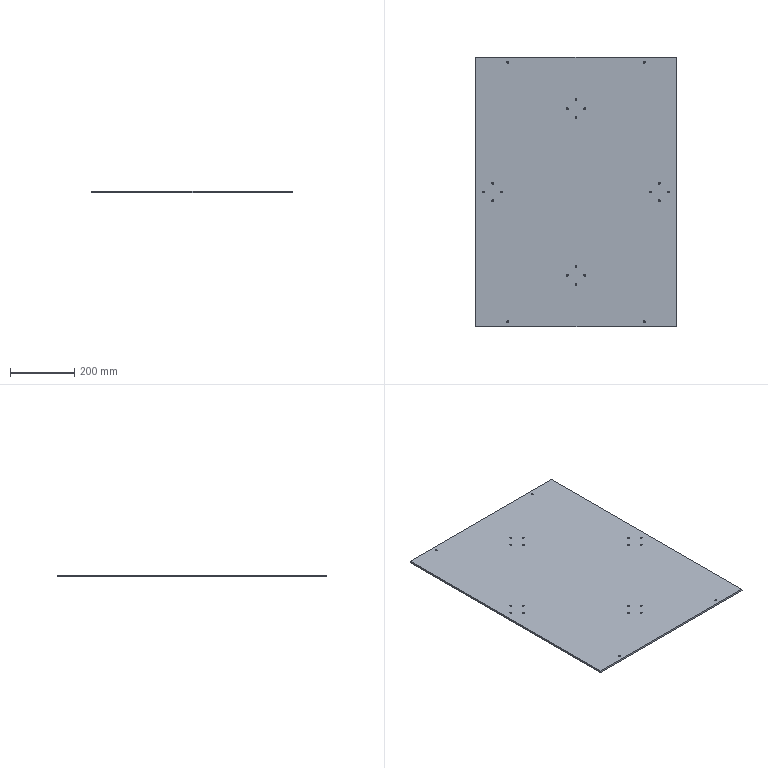Part | SolidWorks | features Cut 2, Extrusion 1 | 1 solid | 62 faces | box 625.685 x 840 x 6 mm | volume 3151419 mm3 | cylinder 40 | plane 22 | commonest cylinder face diameters 6 x40